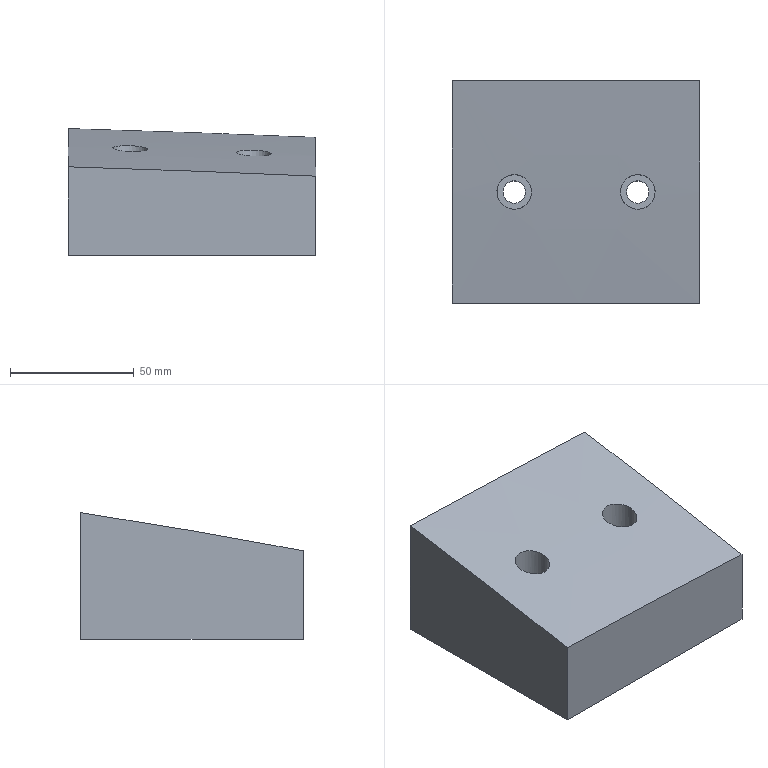Part | NX | features solid 2 | 1 solid | 12 faces | box 100 x 90 x 51.284 mm | volume 369647 mm3 | plane 7 | cylinder 4 | spline 1 | commonest cylinder face diameters 9 x2 14 x2
STEP:
#1=CARTESIAN_POINT('',(359.5,-440.,-110.));
#2=VERTEX_POINT('',#1);
#3=CARTESIAN_POINT('',(355.,-440.,-110.));
#4=DIRECTION('',(0.,0.,1.));
#5=DIRECTION('',(1.,0.,0.));
#6=AXIS2_PLACEMENT_3D('',#3,#4,#5);
#7=CIRCLE('',#6,4.5);
#8=EDGE_CURVE('',#2,#2,#7,.F.);
#9=ORIENTED_EDGE('',*,*,#8,.F.);
#10=EDGE_LOOP('',(#9));
#11=FACE_BOUND('',#10,.T.);
#12=CARTESIAN_POINT('',(430.,-485.,-110.));
#13=VERTEX_POINT('',#12);
#14=CARTESIAN_POINT('',(330.,-485.,-110.));
#15=VERTEX_POINT('',#14);
#16=CARTESIAN_POINT('',(430.,-485.,-110.));
#17=DIRECTION('',(1.,0.,0.));
#18=VECTOR('',#17,1000.);
#19=LINE('',#16,#18);
#20=EDGE_CURVE('',#13,#15,#19,.F.);
#21=ORIENTED_EDGE('',*,*,#20,.T.);
#22=CARTESIAN_POINT('',(330.,-395.,-110.));
#23=VERTEX_POINT('',#22);
#24=CARTESIAN_POINT('',(330.,-485.,-110.));
#25=DIRECTION('',(0.,1.,0.));
#26=VECTOR('',#25,1000.);
#27=LINE('',#24,#26);
#28=EDGE_CURVE('',#15,#23,#27,.T.);
#29=ORIENTED_EDGE('',*,*,#28,.T.);
#30=CARTESIAN_POINT('',(430.,-395.,-110.));
#31=VERTEX_POINT('',#30);
#32=CARTESIAN_POINT('',(430.,-395.,-110.));
#33=DIRECTION('',(1.,0.,0.));
#34=VECTOR('',#33,1000.);
#35=LINE('',#32,#34);
#36=EDGE_CURVE('',#31,#23,#35,.F.);
#37=ORIENTED_EDGE('',*,*,#36,.F.);
#38=CARTESIAN_POINT('',(430.,-485.,-110.));
#39=DIRECTION('',(0.,1.,0.));
#40=VECTOR('',#39,1000.);
#41=LINE('',#38,#40);
#42=EDGE_CURVE('',#13,#31,#41,.T.);
#43=ORIENTED_EDGE('',*,*,#42,.F.);
#44=EDGE_LOOP('',(#21,#29,#37,#43));
#45=FACE_BOUND('',#44,.T.);
#46=CARTESIAN_POINT('',(409.5,-440.,-110.));
#47=VERTEX_POINT('',#46);
#48=CARTESIAN_POINT('',(405.,-440.,-110.));
#49=DIRECTION('',(0.,0.,1.));
#50=DIRECTION('',(1.,0.,0.));
#51=AXIS2_PLACEMENT_3D('',#48,#49,#50);
#52=CIRCLE('',#51,4.5);
#53=EDGE_CURVE('',#47,#47,#52,.F.);
#54=ORIENTED_EDGE('',*,*,#53,.F.);
#55=EDGE_LOOP('',(#54));
#56=FACE_BOUND('',#55,.T.);
#57=CARTESIAN_POINT('',(430.,-485.,-110.));
#58=DIRECTION('',(0.,0.,1.));
#59=DIRECTION('',(0.,1.,0.));
#60=AXIS2_PLACEMENT_3D('',#57,#58,#59);
#61=PLANE('',#60);
#62=ADVANCED_FACE('',(#11,#45,#56),#61,.F.);
#63=CARTESIAN_POINT('',(412.,-440.,-90.));
#64=VERTEX_POINT('',#63);
#65=CARTESIAN_POINT('',(405.,-440.,-90.));
#66=DIRECTION('',(0.,0.,1.));
#67=DIRECTION('',(1.,0.,0.));
#68=AXIS2_PLACEMENT_3D('',#65,#66,#67);
#69=CIRCLE('',#68,7.);
#70=EDGE_CURVE('',#64,#64,#69,.T.);
#71=ORIENTED_EDGE('',*,*,#70,.T.);
#72=EDGE_LOOP('',(#71));
#73=FACE_BOUND('',#72,.T.);
#74=CARTESIAN_POINT('',(400.5,-440.,-90.));
#75=VERTEX_POINT('',#74);
#76=CARTESIAN_POINT('',(405.,-440.,-90.));
#77=DIRECTION('',(0.,0.,-1.));
#78=DIRECTION('',(-1.,0.,0.));
#79=AXIS2_PLACEMENT_3D('',#76,#77,#78);
#80=CIRCLE('',#79,4.5);
#81=EDGE_CURVE('',#75,#75,#80,.F.);
#82=ORIENTED_EDGE('',*,*,#81,.F.);
#83=EDGE_LOOP('',(#82));
#84=FACE_BOUND('',#83,.T.);
#85=CARTESIAN_POINT('',(405.,-440.,-90.));
#86=DIRECTION('',(0.,0.,-1.));
#87=DIRECTION('',(1.,0.,0.));
#88=AXIS2_PLACEMENT_3D('',#85,#86,#87);
#89=PLANE('',#88);
#90=ADVANCED_FACE('',(#73,#84),#89,.F.);
#91=CARTESIAN_POINT('',(362.,-440.,-90.));
#92=VERTEX_POINT('',#91);
#93=CARTESIAN_POINT('',(355.,-440.,-90.));
#94=DIRECTION('',(0.,0.,1.));
#95=DIRECTION('',(1.,0.,0.));
#96=AXIS2_PLACEMENT_3D('',#93,#94,#95);
#97=CIRCLE('',#96,7.);
#98=EDGE_CURVE('',#92,#92,#97,.T.);
#99=ORIENTED_EDGE('',*,*,#98,.T.);
#100=EDGE_LOOP('',(#99));
#101=FACE_BOUND('',#100,.T.);
#102=CARTESIAN_POINT('',(350.5,-440.,-90.));
#103=VERTEX_POINT('',#102);
#104=CARTESIAN_POINT('',(355.,-440.,-90.));
#105=DIRECTION('',(0.,0.,-1.));
#106=DIRECTION('',(-1.,0.,0.));
#107=AXIS2_PLACEMENT_3D('',#104,#105,#106);
#108=CIRCLE('',#107,4.5);
#109=EDGE_CURVE('',#103,#103,#108,.F.);
#110=ORIENTED_EDGE('',*,*,#109,.F.);
#111=EDGE_LOOP('',(#110));
#112=FACE_BOUND('',#111,.T.);
#113=CARTESIAN_POINT('',(355.,-440.,-90.));
#114=DIRECTION('',(0.,0.,-1.));
#115=DIRECTION('',(1.,0.,0.));
#116=AXIS2_PLACEMENT_3D('',#113,#114,#115);
#117=PLANE('',#116);
#118=ADVANCED_FACE('',(#101,#112),#117,.F.);
#119=CARTESIAN_POINT('',(412.,-440.,-68.928));
#120=VERTEX_POINT('',#119);
#121=CARTESIAN_POINT('',(410.515,-434.552,-67.927));
#122=CARTESIAN_POINT('',(412.744,-439.995,-68.956));
#123=CARTESIAN_POINT('',(410.509,-445.469,-69.82));
#124=CARTESIAN_POINT('',(404.974,-447.772,-70.001));
#125=CARTESIAN_POINT('',(399.483,-445.445,-69.372));
#126=CARTESIAN_POINT('',(397.259,-440.01,-68.338));
#127=CARTESIAN_POINT('',(399.482,-434.539,-67.485));
#128=CARTESIAN_POINT('',(405.023,-432.227,-67.31));
#129=CARTESIAN_POINT('',(410.515,-434.552,-67.927));
#130=CARTESIAN_POINT('',(412.744,-439.995,-68.956));
#131=CARTESIAN_POINT('',(410.509,-445.469,-69.82));
#132=B_SPLINE_CURVE_WITH_KNOTS('',3,(#121,#122,#123,#124,#125,#126,#127,#128,#129,#130,#131),.UNSPECIFIED.,.T.,.F.,(1,1,1,1,1,1,1,1,1,1,1,1,1,1,1),(-0.01654,-0.01103,-0.005513,0.,0.005513,0.01103,0.01654,0.02205,0.02757,0.03308,0.03859,0.04411,0.04962,0.05513,0.06065),.UNSPECIFIED.);
#133=EDGE_CURVE('',#120,#120,#132,.T.);
#134=ORIENTED_EDGE('',*,*,#133,.T.);
#135=EDGE_LOOP('',(#134));
#136=FACE_BOUND('',#135,.T.);
#137=CARTESIAN_POINT('',(362.,-440.,-67.058));
#138=VERTEX_POINT('',#137);
#139=CARTESIAN_POINT('',(360.514,-434.549,-66.074));
#140=CARTESIAN_POINT('',(362.744,-439.996,-67.081));
#141=CARTESIAN_POINT('',(360.51,-445.466,-67.953));
#142=CARTESIAN_POINT('',(354.981,-447.772,-68.172));
#143=CARTESIAN_POINT('',(349.483,-445.447,-67.586));
#144=CARTESIAN_POINT('',(347.259,-440.009,-66.574));
#145=CARTESIAN_POINT('',(349.481,-434.542,-65.712));
#146=CARTESIAN_POINT('',(355.016,-432.227,-65.5));
#147=CARTESIAN_POINT('',(360.514,-434.549,-66.074));
#148=CARTESIAN_POINT('',(362.744,-439.996,-67.081));
#149=CARTESIAN_POINT('',(360.51,-445.466,-67.953));
#150=B_SPLINE_CURVE_WITH_KNOTS('',3,(#139,#140,#141,#142,#143,#144,#145,#146,#147,#148,#149),.UNSPECIFIED.,.T.,.F.,(1,1,1,1,1,1,1,1,1,1,1,1,1,1,1),(-0.01654,-0.01102,-0.005512,0.,0.005512,0.01102,0.01654,0.02205,0.02756,0.03307,0.03858,0.04409,0.04961,0.05512,0.06063),.UNSPECIFIED.);
#151=EDGE_CURVE('',#138,#138,#150,.T.);
#152=ORIENTED_EDGE('',*,*,#151,.T.);
#153=EDGE_LOOP('',(#152));
#154=FACE_BOUND('',#153,.T.);
#155=CARTESIAN_POINT('',(430.,-395.,-62.272));
#156=VERTEX_POINT('',#155);
#157=CARTESIAN_POINT('',(330.,-395.,-58.716));
#158=VERTEX_POINT('',#157);
#159=CARTESIAN_POINT('',(430.,-395.,-62.272));
#160=CARTESIAN_POINT('',(396.678,-395.,-60.842));
#161=CARTESIAN_POINT('',(363.34,-395.,-59.677));
#162=CARTESIAN_POINT('',(330.,-395.,-58.716));
#163=B_SPLINE_CURVE_WITH_KNOTS('',3,(#159,#160,#161,#162),.UNSPECIFIED.,.F.,.F.,(4,4),(0.1525,0.2526),.UNSPECIFIED.);
#164=EDGE_CURVE('',#156,#158,#163,.T.);
#165=ORIENTED_EDGE('',*,*,#164,.T.);
#166=CARTESIAN_POINT('',(330.,-485.,-74.159));
#167=VERTEX_POINT('',#166);
#168=CARTESIAN_POINT('',(330.,-485.,-74.159));
#169=CARTESIAN_POINT('',(330.,-455.089,-68.492));
#170=CARTESIAN_POINT('',(330.,-425.086,-63.364));
#171=CARTESIAN_POINT('',(330.,-395.,-58.716));
#172=B_SPLINE_CURVE_WITH_KNOTS('',3,(#168,#169,#170,#171),.UNSPECIFIED.,.F.,.F.,(4,4),(0.,0.09132),.UNSPECIFIED.);
#173=EDGE_CURVE('',#167,#158,#172,.T.);
#174=ORIENTED_EDGE('',*,*,#173,.F.);
#175=CARTESIAN_POINT('',(430.,-485.,-77.949));
#176=VERTEX_POINT('',#175);
#177=CARTESIAN_POINT('',(430.,-485.,-77.949));
#178=CARTESIAN_POINT('',(396.68,-485.,-76.428));
#179=CARTESIAN_POINT('',(363.341,-485.,-75.185));
#180=CARTESIAN_POINT('',(330.,-485.,-74.159));
#181=B_SPLINE_CURVE_WITH_KNOTS('',3,(#177,#178,#179,#180),.UNSPECIFIED.,.F.,.F.,(4,4),(0.3891,0.4891),.UNSPECIFIED.);
#182=EDGE_CURVE('',#176,#167,#181,.T.);
#183=ORIENTED_EDGE('',*,*,#182,.F.);
#184=CARTESIAN_POINT('',(430.,-485.,-77.949));
#185=CARTESIAN_POINT('',(430.,-455.104,-72.176));
#186=CARTESIAN_POINT('',(430.,-425.087,-66.97));
#187=CARTESIAN_POINT('',(430.,-395.,-62.272));
#188=B_SPLINE_CURVE_WITH_KNOTS('',3,(#184,#185,#186,#187),.UNSPECIFIED.,.F.,.F.,(4,4),(0.5019,0.5932),.UNSPECIFIED.);
#189=EDGE_CURVE('',#176,#156,#188,.T.);
#190=ORIENTED_EDGE('',*,*,#189,.T.);
#191=EDGE_LOOP('',(#165,#174,#183,#190));
#192=FACE_BOUND('',#191,.T.);
#193=CARTESIAN_POINT('',(430.601,-394.013,-62.144));
#194=CARTESIAN_POINT('',(396.869,-394.192,-60.722));
#195=CARTESIAN_POINT('',(363.131,-394.338,-59.567));
#196=CARTESIAN_POINT('',(329.388,-394.458,-58.615));
#197=CARTESIAN_POINT('',(430.599,-424.582,-66.894));
#198=CARTESIAN_POINT('',(396.869,-424.766,-65.454));
#199=CARTESIAN_POINT('',(363.132,-424.916,-64.285));
#200=CARTESIAN_POINT('',(329.389,-425.039,-63.322));
#201=CARTESIAN_POINT('',(430.601,-455.09,-72.206));
#202=CARTESIAN_POINT('',(396.872,-455.28,-70.739));
#203=CARTESIAN_POINT('',(363.135,-455.435,-69.546));
#204=CARTESIAN_POINT('',(329.393,-455.563,-68.563));
#205=CARTESIAN_POINT('',(430.605,-485.538,-78.081));
#206=CARTESIAN_POINT('',(396.877,-485.735,-76.575));
#207=CARTESIAN_POINT('',(363.142,-485.897,-75.348));
#208=CARTESIAN_POINT('',(329.4,-486.031,-74.336));
#209=B_SPLINE_SURFACE_WITH_KNOTS('',3,3,((#193,#194,#195,#196),(#197,#198,#199,#200),(#201,#202,#203,#204),(#205,#206,#207,#208)),.UNSPECIFIED.,.F.,.F.,.F.,(4,4),(4,4),(0.6766,0.891),(0.3701,0.4911),.UNSPECIFIED.);
#210=ADVANCED_FACE('',(#136,#154,#192),#209,.F.);
#211=ORIENTED_EDGE('',*,*,#182,.T.);
#212=CARTESIAN_POINT('',(330.,-485.,-60.));
#213=DIRECTION('',(0.,0.,1.));
#214=VECTOR('',#213,1000.);
#215=LINE('',#212,#214);
#216=EDGE_CURVE('',#167,#15,#215,.F.);
#217=ORIENTED_EDGE('',*,*,#216,.T.);
#218=ORIENTED_EDGE('',*,*,#20,.F.);
#219=CARTESIAN_POINT('',(430.,-485.,-60.));
#220=DIRECTION('',(0.,0.,-1.));
#221=VECTOR('',#220,1000.);
#222=LINE('',#219,#221);
#223=EDGE_CURVE('',#176,#13,#222,.T.);
#224=ORIENTED_EDGE('',*,*,#223,.F.);
#225=EDGE_LOOP('',(#211,#217,#218,#224));
#226=FACE_BOUND('',#225,.T.);
#227=CARTESIAN_POINT('',(430.,-485.,-60.));
#228=DIRECTION('',(0.,1.,0.));
#229=DIRECTION('',(0.,0.,-1.));
#230=AXIS2_PLACEMENT_3D('',#227,#228,#229);
#231=PLANE('',#230);
#232=ADVANCED_FACE('',(#226),#231,.F.);
#233=CARTESIAN_POINT('',(430.,-395.,-60.));
#234=DIRECTION('',(0.,0.,-1.));
#235=VECTOR('',#234,1000.);
#236=LINE('',#233,#235);
#237=EDGE_CURVE('',#156,#31,#236,.T.);
#238=ORIENTED_EDGE('',*,*,#237,.T.);
#239=ORIENTED_EDGE('',*,*,#36,.T.);
#240=CARTESIAN_POINT('',(330.,-395.,-60.));
#241=DIRECTION('',(0.,0.,1.));
#242=VECTOR('',#241,1000.);
#243=LINE('',#240,#242);
#244=EDGE_CURVE('',#158,#23,#243,.F.);
#245=ORIENTED_EDGE('',*,*,#244,.F.);
#246=ORIENTED_EDGE('',*,*,#164,.F.);
#247=EDGE_LOOP('',(#238,#239,#245,#246));
#248=FACE_BOUND('',#247,.T.);
#249=CARTESIAN_POINT('',(430.,-395.,-60.));
#250=DIRECTION('',(0.,1.,0.));
#251=DIRECTION('',(0.,0.,-1.));
#252=AXIS2_PLACEMENT_3D('',#249,#250,#251);
#253=PLANE('',#252);
#254=ADVANCED_FACE('',(#248),#253,.T.);
#255=ORIENTED_EDGE('',*,*,#28,.F.);
#256=ORIENTED_EDGE('',*,*,#216,.F.);
#257=ORIENTED_EDGE('',*,*,#173,.T.);
#258=ORIENTED_EDGE('',*,*,#244,.T.);
#259=EDGE_LOOP('',(#255,#256,#257,#258));
#260=FACE_BOUND('',#259,.T.);
#261=CARTESIAN_POINT('',(330.,-485.,-60.));
#262=DIRECTION('',(-1.,0.,0.));
#263=DIRECTION('',(0.,0.,1.));
#264=AXIS2_PLACEMENT_3D('',#261,#262,#263);
#265=PLANE('',#264);
#266=ADVANCED_FACE('',(#260),#265,.T.);
#267=ORIENTED_EDGE('',*,*,#42,.T.);
#268=ORIENTED_EDGE('',*,*,#237,.F.);
#269=ORIENTED_EDGE('',*,*,#189,.F.);
#270=ORIENTED_EDGE('',*,*,#223,.T.);
#271=EDGE_LOOP('',(#267,#268,#269,#270));
#272=FACE_BOUND('',#271,.T.);
#273=CARTESIAN_POINT('',(430.,-485.,-60.));
#274=DIRECTION('',(-1.,0.,0.));
#275=DIRECTION('',(0.,0.,1.));
#276=AXIS2_PLACEMENT_3D('',#273,#274,#275);
#277=PLANE('',#276);
#278=ADVANCED_FACE('',(#272),#277,.F.);
#279=ORIENTED_EDGE('',*,*,#98,.F.);
#280=EDGE_LOOP('',(#279));
#281=FACE_BOUND('',#280,.T.);
#282=ORIENTED_EDGE('',*,*,#151,.F.);
#283=EDGE_LOOP('',(#282));
#284=FACE_BOUND('',#283,.T.);
#285=CARTESIAN_POINT('',(355.,-440.,410.));
#286=DIRECTION('',(0.,0.,-1.));
#287=DIRECTION('',(1.,0.,0.));
#288=AXIS2_PLACEMENT_3D('',#285,#286,#287);
#289=CYLINDRICAL_SURFACE('',#288,7.);
#290=ADVANCED_FACE('',(#281,#284),#289,.F.);
#291=ORIENTED_EDGE('',*,*,#70,.F.);
#292=EDGE_LOOP('',(#291));
#293=FACE_BOUND('',#292,.T.);
#294=ORIENTED_EDGE('',*,*,#133,.F.);
#295=EDGE_LOOP('',(#294));
#296=FACE_BOUND('',#295,.T.);
#297=CARTESIAN_POINT('',(405.,-440.,410.));
#298=DIRECTION('',(0.,0.,-1.));
#299=DIRECTION('',(1.,0.,0.));
#300=AXIS2_PLACEMENT_3D('',#297,#298,#299);
#301=CYLINDRICAL_SURFACE('',#300,7.);
#302=ADVANCED_FACE('',(#293,#296),#301,.F.);
#303=ORIENTED_EDGE('',*,*,#109,.T.);
#304=EDGE_LOOP('',(#303));
#305=FACE_BOUND('',#304,.T.);
#306=ORIENTED_EDGE('',*,*,#8,.T.);
#307=EDGE_LOOP('',(#306));
#308=FACE_BOUND('',#307,.T.);
#309=CARTESIAN_POINT('',(355.,-440.,375.));
#310=DIRECTION('',(0.,0.,-1.));
#311=DIRECTION('',(-1.,0.,0.));
#312=AXIS2_PLACEMENT_3D('',#309,#310,#311);
#313=CYLINDRICAL_SURFACE('',#312,4.5);
#314=ADVANCED_FACE('',(#305,#308),#313,.F.);
#315=ORIENTED_EDGE('',*,*,#81,.T.);
#316=EDGE_LOOP('',(#315));
#317=FACE_BOUND('',#316,.T.);
#318=ORIENTED_EDGE('',*,*,#53,.T.);
#319=EDGE_LOOP('',(#318));
#320=FACE_BOUND('',#319,.T.);
#321=CARTESIAN_POINT('',(405.,-440.,375.));
#322=DIRECTION('',(0.,0.,-1.));
#323=DIRECTION('',(-1.,0.,0.));
#324=AXIS2_PLACEMENT_3D('',#321,#322,#323);
#325=CYLINDRICAL_SURFACE('',#324,4.5);
#326=ADVANCED_FACE('',(#317,#320),#325,.F.);
#327=CLOSED_SHELL('',(#62,#90,#118,#210,#232,#254,#266,#278,#290,#302,#314,#326));
#328=MANIFOLD_SOLID_BREP('',#327);
#329=(LENGTH_UNIT()NAMED_UNIT(*)SI_UNIT(.MILLI.,.METRE.));
#330=UNCERTAINTY_MEASURE_WITH_UNIT(LENGTH_MEASURE(0.0508),#329,'','');
#331=(NAMED_UNIT(*)PLANE_ANGLE_UNIT()SI_UNIT($,.RADIAN.));
#332=(NAMED_UNIT(*)SI_UNIT($,.STERADIAN.)SOLID_ANGLE_UNIT());
#333=(GEOMETRIC_REPRESENTATION_CONTEXT(3)GLOBAL_UNCERTAINTY_ASSIGNED_CONTEXT((#330))GLOBAL_UNIT_ASSIGNED_CONTEXT((#329,#331,#332))REPRESENTATION_CONTEXT('',''));
#334=ADVANCED_BREP_SHAPE_REPRESENTATION('',(#328),#333);